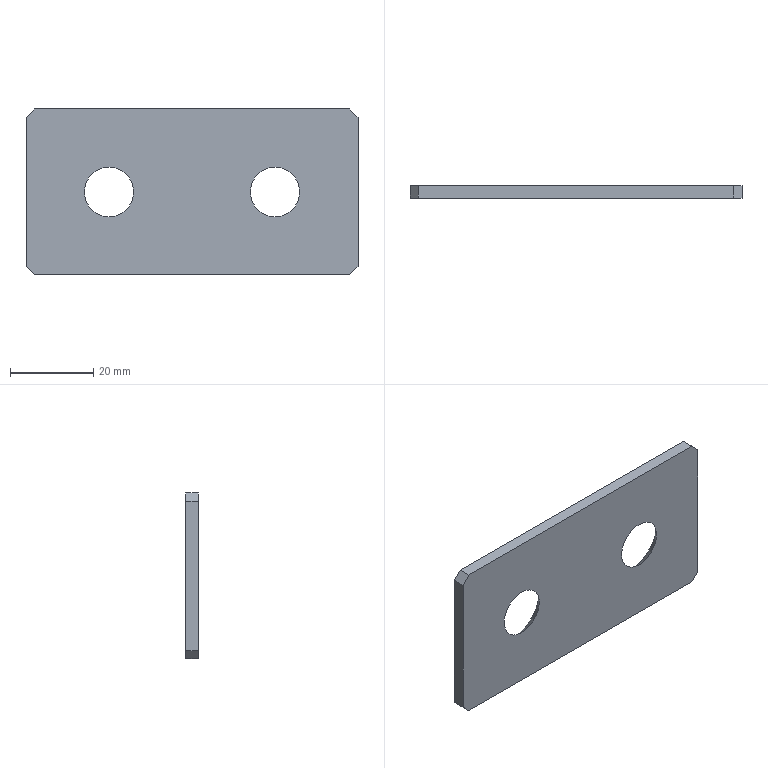Part | NX | 1 solid | 12 faces | box 80 x 3 x 40 mm | volume 8513 mm3 | plane 10 | cone 2
STEP:
#1=CARTESIAN_POINT('',(20.,-3.,5.96));
#2=VERTEX_POINT('',#1);
#3=CARTESIAN_POINT('',(20.,-3.,0.));
#4=DIRECTION('',(0.,1.,0.));
#5=DIRECTION('',(0.,0.,1.));
#6=AXIS2_PLACEMENT_3D('',#3,#4,#5);
#7=CIRCLE('',#6,5.96);
#8=EDGE_CURVE('',#2,#2,#7,.T.);
#9=ORIENTED_EDGE('',*,*,#8,.T.);
#10=EDGE_LOOP('',(#9));
#11=FACE_BOUND('',#10,.T.);
#12=CARTESIAN_POINT('',(0.,-3.,18.));
#13=VERTEX_POINT('',#12);
#14=CARTESIAN_POINT('',(0.,-3.,-18.));
#15=VERTEX_POINT('',#14);
#16=CARTESIAN_POINT('',(0.,-3.,20.));
#17=DIRECTION('',(0.,0.,-1.));
#18=VECTOR('',#17,1000.);
#19=LINE('',#16,#18);
#20=EDGE_CURVE('',#13,#15,#19,.T.);
#21=ORIENTED_EDGE('',*,*,#20,.T.);
#22=CARTESIAN_POINT('',(2.,-3.,-20.));
#23=VERTEX_POINT('',#22);
#24=CARTESIAN_POINT('',(2.,-3.,-20.));
#25=DIRECTION('',(-0.7071,0.,0.7071));
#26=VECTOR('',#25,1000.);
#27=LINE('',#24,#26);
#28=EDGE_CURVE('',#15,#23,#27,.F.);
#29=ORIENTED_EDGE('',*,*,#28,.T.);
#30=CARTESIAN_POINT('',(78.,-3.,-20.));
#31=VERTEX_POINT('',#30);
#32=CARTESIAN_POINT('',(0.,-3.,-20.));
#33=DIRECTION('',(1.,0.,0.));
#34=VECTOR('',#33,1000.);
#35=LINE('',#32,#34);
#36=EDGE_CURVE('',#23,#31,#35,.T.);
#37=ORIENTED_EDGE('',*,*,#36,.T.);
#38=CARTESIAN_POINT('',(80.,-3.,-18.));
#39=VERTEX_POINT('',#38);
#40=CARTESIAN_POINT('',(78.,-3.,-20.));
#41=DIRECTION('',(-0.7071,0.,-0.7071));
#42=VECTOR('',#41,1000.);
#43=LINE('',#40,#42);
#44=EDGE_CURVE('',#31,#39,#43,.F.);
#45=ORIENTED_EDGE('',*,*,#44,.T.);
#46=CARTESIAN_POINT('',(80.,-3.,18.));
#47=VERTEX_POINT('',#46);
#48=CARTESIAN_POINT('',(80.,-3.,20.));
#49=DIRECTION('',(0.,0.,-1.));
#50=VECTOR('',#49,1000.);
#51=LINE('',#48,#50);
#52=EDGE_CURVE('',#47,#39,#51,.T.);
#53=ORIENTED_EDGE('',*,*,#52,.F.);
#54=CARTESIAN_POINT('',(78.,-3.,20.));
#55=VERTEX_POINT('',#54);
#56=CARTESIAN_POINT('',(80.,-3.,18.));
#57=DIRECTION('',(-0.7071,0.,0.7071));
#58=VECTOR('',#57,1000.);
#59=LINE('',#56,#58);
#60=EDGE_CURVE('',#47,#55,#59,.T.);
#61=ORIENTED_EDGE('',*,*,#60,.T.);
#62=CARTESIAN_POINT('',(2.,-3.,20.));
#63=VERTEX_POINT('',#62);
#64=CARTESIAN_POINT('',(0.,-3.,20.));
#65=DIRECTION('',(1.,0.,0.));
#66=VECTOR('',#65,1000.);
#67=LINE('',#64,#66);
#68=EDGE_CURVE('',#63,#55,#67,.T.);
#69=ORIENTED_EDGE('',*,*,#68,.F.);
#70=CARTESIAN_POINT('',(0.,-3.,18.));
#71=DIRECTION('',(-0.7071,0.,-0.7071));
#72=VECTOR('',#71,1000.);
#73=LINE('',#70,#72);
#74=EDGE_CURVE('',#63,#13,#73,.T.);
#75=ORIENTED_EDGE('',*,*,#74,.T.);
#76=EDGE_LOOP('',(#21,#29,#37,#45,#53,#61,#69,#75));
#77=FACE_BOUND('',#76,.T.);
#78=CARTESIAN_POINT('',(60.,-3.,5.96));
#79=VERTEX_POINT('',#78);
#80=CARTESIAN_POINT('',(60.,-3.,0.));
#81=DIRECTION('',(0.,1.,0.));
#82=DIRECTION('',(0.,0.,1.));
#83=AXIS2_PLACEMENT_3D('',#80,#81,#82);
#84=CIRCLE('',#83,5.96);
#85=EDGE_CURVE('',#79,#79,#84,.T.);
#86=ORIENTED_EDGE('',*,*,#85,.T.);
#87=EDGE_LOOP('',(#86));
#88=FACE_BOUND('',#87,.T.);
#89=CARTESIAN_POINT('',(0.,-3.,20.));
#90=DIRECTION('',(0.,1.,0.));
#91=DIRECTION('',(0.,0.,1.));
#92=AXIS2_PLACEMENT_3D('',#89,#90,#91);
#93=PLANE('',#92);
#94=ADVANCED_FACE('',(#11,#77,#88),#93,.F.);
#95=ORIENTED_EDGE('',*,*,#52,.T.);
#96=CARTESIAN_POINT('',(80.,0.,-18.));
#97=VERTEX_POINT('',#96);
#98=CARTESIAN_POINT('',(80.,0.,-18.));
#99=DIRECTION('',(0.,1.,0.));
#100=VECTOR('',#99,1000.);
#101=LINE('',#98,#100);
#102=EDGE_CURVE('',#39,#97,#101,.T.);
#103=ORIENTED_EDGE('',*,*,#102,.T.);
#104=CARTESIAN_POINT('',(80.,0.,18.));
#105=VERTEX_POINT('',#104);
#106=CARTESIAN_POINT('',(80.,0.,20.));
#107=DIRECTION('',(0.,0.,-1.));
#108=VECTOR('',#107,1000.);
#109=LINE('',#106,#108);
#110=EDGE_CURVE('',#105,#97,#109,.T.);
#111=ORIENTED_EDGE('',*,*,#110,.F.);
#112=CARTESIAN_POINT('',(80.,-3.,18.));
#113=DIRECTION('',(0.,-1.,0.));
#114=VECTOR('',#113,1000.);
#115=LINE('',#112,#114);
#116=EDGE_CURVE('',#105,#47,#115,.T.);
#117=ORIENTED_EDGE('',*,*,#116,.T.);
#118=EDGE_LOOP('',(#95,#103,#111,#117));
#119=FACE_BOUND('',#118,.T.);
#120=CARTESIAN_POINT('',(80.,0.,20.));
#121=DIRECTION('',(1.,0.,0.));
#122=DIRECTION('',(0.,0.,-1.));
#123=AXIS2_PLACEMENT_3D('',#120,#121,#122);
#124=PLANE('',#123);
#125=ADVANCED_FACE('',(#119),#124,.T.);
#126=CARTESIAN_POINT('',(20.,0.,8.96));
#127=VERTEX_POINT('',#126);
#128=CARTESIAN_POINT('',(20.,0.,0.));
#129=DIRECTION('',(0.,1.,0.));
#130=DIRECTION('',(0.,0.,1.));
#131=AXIS2_PLACEMENT_3D('',#128,#129,#130);
#132=CIRCLE('',#131,8.96);
#133=EDGE_CURVE('',#127,#127,#132,.T.);
#134=ORIENTED_EDGE('',*,*,#133,.F.);
#135=EDGE_LOOP('',(#134));
#136=FACE_BOUND('',#135,.T.);
#137=CARTESIAN_POINT('',(60.,0.,8.96));
#138=VERTEX_POINT('',#137);
#139=CARTESIAN_POINT('',(60.,0.,0.));
#140=DIRECTION('',(0.,1.,0.));
#141=DIRECTION('',(0.,0.,1.));
#142=AXIS2_PLACEMENT_3D('',#139,#140,#141);
#143=CIRCLE('',#142,8.96);
#144=EDGE_CURVE('',#138,#138,#143,.T.);
#145=ORIENTED_EDGE('',*,*,#144,.F.);
#146=EDGE_LOOP('',(#145));
#147=FACE_BOUND('',#146,.T.);
#148=CARTESIAN_POINT('',(2.,0.,-20.));
#149=VERTEX_POINT('',#148);
#150=CARTESIAN_POINT('',(78.,0.,-20.));
#151=VERTEX_POINT('',#150);
#152=CARTESIAN_POINT('',(0.,0.,-20.));
#153=DIRECTION('',(1.,0.,0.));
#154=VECTOR('',#153,1000.);
#155=LINE('',#152,#154);
#156=EDGE_CURVE('',#149,#151,#155,.T.);
#157=ORIENTED_EDGE('',*,*,#156,.F.);
#158=CARTESIAN_POINT('',(0.,0.,-18.));
#159=VERTEX_POINT('',#158);
#160=CARTESIAN_POINT('',(-19.,0.,1.));
#161=DIRECTION('',(0.7071,0.,-0.7071));
#162=VECTOR('',#161,1000.);
#163=LINE('',#160,#162);
#164=EDGE_CURVE('',#149,#159,#163,.F.);
#165=ORIENTED_EDGE('',*,*,#164,.T.);
#166=CARTESIAN_POINT('',(0.,0.,18.));
#167=VERTEX_POINT('',#166);
#168=CARTESIAN_POINT('',(0.,0.,20.));
#169=DIRECTION('',(0.,0.,-1.));
#170=VECTOR('',#169,1000.);
#171=LINE('',#168,#170);
#172=EDGE_CURVE('',#167,#159,#171,.T.);
#173=ORIENTED_EDGE('',*,*,#172,.F.);
#174=CARTESIAN_POINT('',(2.,0.,20.));
#175=VERTEX_POINT('',#174);
#176=CARTESIAN_POINT('',(1.,0.,19.));
#177=DIRECTION('',(0.7071,0.,0.7071));
#178=VECTOR('',#177,1000.);
#179=LINE('',#176,#178);
#180=EDGE_CURVE('',#167,#175,#179,.T.);
#181=ORIENTED_EDGE('',*,*,#180,.T.);
#182=CARTESIAN_POINT('',(78.,0.,20.));
#183=VERTEX_POINT('',#182);
#184=CARTESIAN_POINT('',(0.,0.,20.));
#185=DIRECTION('',(1.,0.,0.));
#186=VECTOR('',#185,1000.);
#187=LINE('',#184,#186);
#188=EDGE_CURVE('',#175,#183,#187,.T.);
#189=ORIENTED_EDGE('',*,*,#188,.T.);
#190=CARTESIAN_POINT('',(39.,0.,59.));
#191=DIRECTION('',(0.7071,0.,-0.7071));
#192=VECTOR('',#191,1000.);
#193=LINE('',#190,#192);
#194=EDGE_CURVE('',#183,#105,#193,.T.);
#195=ORIENTED_EDGE('',*,*,#194,.T.);
#196=ORIENTED_EDGE('',*,*,#110,.T.);
#197=CARTESIAN_POINT('',(59.,0.,-39.));
#198=DIRECTION('',(0.7071,0.,0.7071));
#199=VECTOR('',#198,1000.);
#200=LINE('',#197,#199);
#201=EDGE_CURVE('',#97,#151,#200,.F.);
#202=ORIENTED_EDGE('',*,*,#201,.T.);
#203=EDGE_LOOP('',(#157,#165,#173,#181,#189,#195,#196,#202));
#204=FACE_BOUND('',#203,.T.);
#205=CARTESIAN_POINT('',(0.,0.,20.));
#206=DIRECTION('',(0.,1.,0.));
#207=DIRECTION('',(0.,0.,1.));
#208=AXIS2_PLACEMENT_3D('',#205,#206,#207);
#209=PLANE('',#208);
#210=ADVANCED_FACE('',(#136,#147,#204),#209,.T.);
#211=ORIENTED_EDGE('',*,*,#172,.T.);
#212=CARTESIAN_POINT('',(0.,-3.,-18.));
#213=DIRECTION('',(0.,-1.,0.));
#214=VECTOR('',#213,1000.);
#215=LINE('',#212,#214);
#216=EDGE_CURVE('',#159,#15,#215,.T.);
#217=ORIENTED_EDGE('',*,*,#216,.T.);
#218=ORIENTED_EDGE('',*,*,#20,.F.);
#219=CARTESIAN_POINT('',(0.,0.,18.));
#220=DIRECTION('',(0.,1.,0.));
#221=VECTOR('',#220,1000.);
#222=LINE('',#219,#221);
#223=EDGE_CURVE('',#13,#167,#222,.T.);
#224=ORIENTED_EDGE('',*,*,#223,.T.);
#225=EDGE_LOOP('',(#211,#217,#218,#224));
#226=FACE_BOUND('',#225,.T.);
#227=CARTESIAN_POINT('',(0.,-3.,20.));
#228=DIRECTION('',(-1.,0.,0.));
#229=DIRECTION('',(0.,0.,1.));
#230=AXIS2_PLACEMENT_3D('',#227,#228,#229);
#231=PLANE('',#230);
#232=ADVANCED_FACE('',(#226),#231,.T.);
#233=ORIENTED_EDGE('',*,*,#188,.F.);
#234=CARTESIAN_POINT('',(2.,-3.,20.));
#235=DIRECTION('',(0.,-1.,0.));
#236=VECTOR('',#235,1000.);
#237=LINE('',#234,#236);
#238=EDGE_CURVE('',#175,#63,#237,.T.);
#239=ORIENTED_EDGE('',*,*,#238,.T.);
#240=ORIENTED_EDGE('',*,*,#68,.T.);
#241=CARTESIAN_POINT('',(78.,0.,20.));
#242=DIRECTION('',(0.,1.,0.));
#243=VECTOR('',#242,1000.);
#244=LINE('',#241,#243);
#245=EDGE_CURVE('',#55,#183,#244,.T.);
#246=ORIENTED_EDGE('',*,*,#245,.T.);
#247=EDGE_LOOP('',(#233,#239,#240,#246));
#248=FACE_BOUND('',#247,.T.);
#249=CARTESIAN_POINT('',(0.,0.,20.));
#250=DIRECTION('',(0.,0.,-1.));
#251=DIRECTION('',(-1.,0.,0.));
#252=AXIS2_PLACEMENT_3D('',#249,#250,#251);
#253=PLANE('',#252);
#254=ADVANCED_FACE('',(#248),#253,.F.);
#255=ORIENTED_EDGE('',*,*,#36,.F.);
#256=CARTESIAN_POINT('',(2.,0.,-20.));
#257=DIRECTION('',(0.,1.,0.));
#258=VECTOR('',#257,1000.);
#259=LINE('',#256,#258);
#260=EDGE_CURVE('',#23,#149,#259,.T.);
#261=ORIENTED_EDGE('',*,*,#260,.T.);
#262=ORIENTED_EDGE('',*,*,#156,.T.);
#263=CARTESIAN_POINT('',(78.,0.,-20.));
#264=DIRECTION('',(0.,-1.,0.));
#265=VECTOR('',#264,1000.);
#266=LINE('',#263,#265);
#267=EDGE_CURVE('',#151,#31,#266,.T.);
#268=ORIENTED_EDGE('',*,*,#267,.T.);
#269=EDGE_LOOP('',(#255,#261,#262,#268));
#270=FACE_BOUND('',#269,.T.);
#271=CARTESIAN_POINT('',(0.,0.,-20.));
#272=DIRECTION('',(0.,0.,-1.));
#273=DIRECTION('',(-1.,0.,0.));
#274=AXIS2_PLACEMENT_3D('',#271,#272,#273);
#275=PLANE('',#274);
#276=ADVANCED_FACE('',(#270),#275,.T.);
#277=ORIENTED_EDGE('',*,*,#28,.F.);
#278=ORIENTED_EDGE('',*,*,#216,.F.);
#279=ORIENTED_EDGE('',*,*,#164,.F.);
#280=ORIENTED_EDGE('',*,*,#260,.F.);
#281=EDGE_LOOP('',(#277,#278,#279,#280));
#282=FACE_BOUND('',#281,.T.);
#283=CARTESIAN_POINT('',(2.,0.,-20.));
#284=DIRECTION('',(0.7071,0.,0.7071));
#285=DIRECTION('',(0.,1.,0.));
#286=AXIS2_PLACEMENT_3D('',#283,#284,#285);
#287=PLANE('',#286);
#288=ADVANCED_FACE('',(#282),#287,.F.);
#289=ORIENTED_EDGE('',*,*,#74,.F.);
#290=ORIENTED_EDGE('',*,*,#238,.F.);
#291=ORIENTED_EDGE('',*,*,#180,.F.);
#292=ORIENTED_EDGE('',*,*,#223,.F.);
#293=EDGE_LOOP('',(#289,#290,#291,#292));
#294=FACE_BOUND('',#293,.T.);
#295=CARTESIAN_POINT('',(0.,-3.,18.));
#296=DIRECTION('',(-0.7071,0.,0.7071));
#297=DIRECTION('',(0.,-1.,0.));
#298=AXIS2_PLACEMENT_3D('',#295,#296,#297);
#299=PLANE('',#298);
#300=ADVANCED_FACE('',(#294),#299,.T.);
#301=ORIENTED_EDGE('',*,*,#201,.F.);
#302=ORIENTED_EDGE('',*,*,#102,.F.);
#303=ORIENTED_EDGE('',*,*,#44,.F.);
#304=ORIENTED_EDGE('',*,*,#267,.F.);
#305=EDGE_LOOP('',(#301,#302,#303,#304));
#306=FACE_BOUND('',#305,.T.);
#307=CARTESIAN_POINT('',(78.,0.,-20.));
#308=DIRECTION('',(-0.7071,0.,0.7071));
#309=DIRECTION('',(0.,-1.,0.));
#310=AXIS2_PLACEMENT_3D('',#307,#308,#309);
#311=PLANE('',#310);
#312=ADVANCED_FACE('',(#306),#311,.F.);
#313=ORIENTED_EDGE('',*,*,#194,.F.);
#314=ORIENTED_EDGE('',*,*,#245,.F.);
#315=ORIENTED_EDGE('',*,*,#60,.F.);
#316=ORIENTED_EDGE('',*,*,#116,.F.);
#317=EDGE_LOOP('',(#313,#314,#315,#316));
#318=FACE_BOUND('',#317,.T.);
#319=CARTESIAN_POINT('',(80.,0.,18.));
#320=DIRECTION('',(0.7071,0.,0.7071));
#321=DIRECTION('',(0.,1.,0.));
#322=AXIS2_PLACEMENT_3D('',#319,#320,#321);
#323=PLANE('',#322);
#324=ADVANCED_FACE('',(#318),#323,.T.);
#325=ORIENTED_EDGE('',*,*,#144,.T.);
#326=EDGE_LOOP('',(#325));
#327=FACE_BOUND('',#326,.T.);
#328=ORIENTED_EDGE('',*,*,#85,.F.);
#329=EDGE_LOOP('',(#328));
#330=FACE_BOUND('',#329,.T.);
#331=CARTESIAN_POINT('',(60.,0.,0.));
#332=DIRECTION('',(0.,1.,0.));
#333=DIRECTION('',(0.,0.,1.));
#334=AXIS2_PLACEMENT_3D('',#331,#332,#333);
#335=CONICAL_SURFACE('',#334,8.96,0.7854);
#336=ADVANCED_FACE('',(#327,#330),#335,.F.);
#337=ORIENTED_EDGE('',*,*,#133,.T.);
#338=EDGE_LOOP('',(#337));
#339=FACE_BOUND('',#338,.T.);
#340=ORIENTED_EDGE('',*,*,#8,.F.);
#341=EDGE_LOOP('',(#340));
#342=FACE_BOUND('',#341,.T.);
#343=CARTESIAN_POINT('',(20.,0.,0.));
#344=DIRECTION('',(0.,1.,0.));
#345=DIRECTION('',(0.,0.,1.));
#346=AXIS2_PLACEMENT_3D('',#343,#344,#345);
#347=CONICAL_SURFACE('',#346,8.96,0.7854);
#348=ADVANCED_FACE('',(#339,#342),#347,.F.);
#349=CLOSED_SHELL('',(#94,#125,#210,#232,#254,#276,#288,#300,#312,#324,#336,#348));
#350=MANIFOLD_SOLID_BREP('',#349);
#351=(LENGTH_UNIT()NAMED_UNIT(*)SI_UNIT(.MILLI.,.METRE.));
#352=UNCERTAINTY_MEASURE_WITH_UNIT(LENGTH_MEASURE(0.00001),#351,'','');
#353=(NAMED_UNIT(*)PLANE_ANGLE_UNIT()SI_UNIT($,.RADIAN.));
#354=(NAMED_UNIT(*)SI_UNIT($,.STERADIAN.)SOLID_ANGLE_UNIT());
#355=(GEOMETRIC_REPRESENTATION_CONTEXT(3)GLOBAL_UNCERTAINTY_ASSIGNED_CONTEXT((#352))GLOBAL_UNIT_ASSIGNED_CONTEXT((#351,#353,#354))REPRESENTATION_CONTEXT('',''));
#356=ADVANCED_BREP_SHAPE_REPRESENTATION('',(#350),#355);